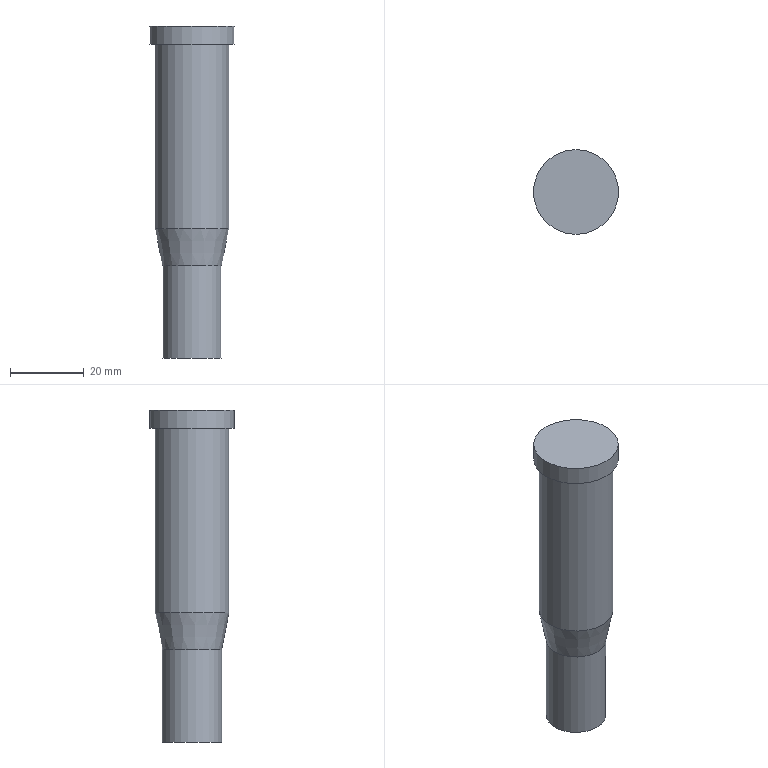Part | NX | features solid 2 | 1 solid | 7 faces | box 23 x 23 x 90 mm | volume 25444 mm3 | plane 3 | cylinder 3 | cone 1 | commonest cylinder face diameters 16.1 x1 20 x1 23 x1
STEP:
#1=CARTESIAN_POINT('',(-384.,15.95,111.));
#2=VERTEX_POINT('',#1);
#3=CARTESIAN_POINT('',(-384.,24.,111.));
#4=DIRECTION('',(0.,0.,1.));
#5=DIRECTION('',(0.,-1.,0.));
#6=AXIS2_PLACEMENT_3D('',#3,#4,#5);
#7=CIRCLE('',#6,8.05);
#8=EDGE_CURVE('',#2,#2,#7,.T.);
#9=ORIENTED_EDGE('',*,*,#8,.F.);
#10=EDGE_LOOP('',(#9));
#11=FACE_BOUND('',#10,.T.);
#12=CARTESIAN_POINT('',(-384.,24.,111.));
#13=DIRECTION('',(0.,0.,-1.));
#14=DIRECTION('',(0.,1.,0.));
#15=AXIS2_PLACEMENT_3D('',#12,#13,#14);
#16=PLANE('',#15);
#17=ADVANCED_FACE('',(#11),#16,.T.);
#18=CARTESIAN_POINT('',(-384.,15.95,136.));
#19=VERTEX_POINT('',#18);
#20=CARTESIAN_POINT('',(-384.,24.,136.));
#21=DIRECTION('',(0.,0.,1.));
#22=DIRECTION('',(0.,-1.,0.));
#23=AXIS2_PLACEMENT_3D('',#20,#21,#22);
#24=CIRCLE('',#23,8.05);
#25=EDGE_CURVE('',#19,#19,#24,.T.);
#26=ORIENTED_EDGE('',*,*,#25,.F.);
#27=EDGE_LOOP('',(#26));
#28=FACE_BOUND('',#27,.T.);
#29=ORIENTED_EDGE('',*,*,#8,.T.);
#30=EDGE_LOOP('',(#29));
#31=FACE_BOUND('',#30,.T.);
#32=CARTESIAN_POINT('',(-384.,24.,111.));
#33=DIRECTION('',(0.,0.,1.));
#34=DIRECTION('',(0.,-1.,0.));
#35=AXIS2_PLACEMENT_3D('',#32,#33,#34);
#36=CYLINDRICAL_SURFACE('',#35,8.05);
#37=ADVANCED_FACE('',(#28,#31),#36,.T.);
#38=ORIENTED_EDGE('',*,*,#25,.T.);
#39=EDGE_LOOP('',(#38));
#40=FACE_BOUND('',#39,.T.);
#41=CARTESIAN_POINT('',(-384.,14.,146.));
#42=VERTEX_POINT('',#41);
#43=CARTESIAN_POINT('',(-384.,24.,146.));
#44=DIRECTION('',(0.,0.,1.));
#45=DIRECTION('',(0.,-1.,0.));
#46=AXIS2_PLACEMENT_3D('',#43,#44,#45);
#47=CIRCLE('',#46,10.);
#48=EDGE_CURVE('',#42,#42,#47,.T.);
#49=ORIENTED_EDGE('',*,*,#48,.F.);
#50=EDGE_LOOP('',(#49));
#51=FACE_BOUND('',#50,.T.);
#52=CARTESIAN_POINT('',(-384.,24.,136.));
#53=DIRECTION('',(0.,0.,1.));
#54=DIRECTION('',(0.,-1.,0.));
#55=AXIS2_PLACEMENT_3D('',#52,#53,#54);
#56=CONICAL_SURFACE('',#55,8.05,0.1926);
#57=ADVANCED_FACE('',(#40,#51),#56,.T.);
#58=CARTESIAN_POINT('',(-384.,34.,196.));
#59=VERTEX_POINT('',#58);
#60=CARTESIAN_POINT('',(-384.,24.,196.));
#61=DIRECTION('',(0.,0.,-1.));
#62=DIRECTION('',(0.,1.,0.));
#63=AXIS2_PLACEMENT_3D('',#60,#61,#62);
#64=CIRCLE('',#63,10.);
#65=EDGE_CURVE('',#59,#59,#64,.F.);
#66=ORIENTED_EDGE('',*,*,#65,.F.);
#67=EDGE_LOOP('',(#66));
#68=FACE_BOUND('',#67,.T.);
#69=ORIENTED_EDGE('',*,*,#48,.T.);
#70=EDGE_LOOP('',(#69));
#71=FACE_BOUND('',#70,.T.);
#72=CARTESIAN_POINT('',(-384.,24.,146.));
#73=DIRECTION('',(0.,0.,1.));
#74=DIRECTION('',(0.,-1.,0.));
#75=AXIS2_PLACEMENT_3D('',#72,#73,#74);
#76=CYLINDRICAL_SURFACE('',#75,10.);
#77=ADVANCED_FACE('',(#68,#71),#76,.T.);
#78=CARTESIAN_POINT('',(-384.,12.5,201.));
#79=VERTEX_POINT('',#78);
#80=CARTESIAN_POINT('',(-384.,24.,201.));
#81=DIRECTION('',(0.,0.,1.));
#82=DIRECTION('',(0.,-1.,0.));
#83=AXIS2_PLACEMENT_3D('',#80,#81,#82);
#84=CIRCLE('',#83,11.5);
#85=EDGE_CURVE('',#79,#79,#84,.F.);
#86=ORIENTED_EDGE('',*,*,#85,.F.);
#87=EDGE_LOOP('',(#86));
#88=FACE_BOUND('',#87,.T.);
#89=CARTESIAN_POINT('',(-384.,24.,201.));
#90=DIRECTION('',(0.,0.,1.));
#91=DIRECTION('',(0.,-1.,0.));
#92=AXIS2_PLACEMENT_3D('',#89,#90,#91);
#93=PLANE('',#92);
#94=ADVANCED_FACE('',(#88),#93,.T.);
#95=ORIENTED_EDGE('',*,*,#65,.T.);
#96=EDGE_LOOP('',(#95));
#97=FACE_BOUND('',#96,.T.);
#98=CARTESIAN_POINT('',(-384.,35.5,196.));
#99=VERTEX_POINT('',#98);
#100=CARTESIAN_POINT('',(-384.,24.,196.));
#101=DIRECTION('',(0.,0.,-1.));
#102=DIRECTION('',(0.,1.,0.));
#103=AXIS2_PLACEMENT_3D('',#100,#101,#102);
#104=CIRCLE('',#103,11.5);
#105=EDGE_CURVE('',#99,#99,#104,.F.);
#106=ORIENTED_EDGE('',*,*,#105,.F.);
#107=EDGE_LOOP('',(#106));
#108=FACE_BOUND('',#107,.T.);
#109=CARTESIAN_POINT('',(-384.,24.,196.));
#110=DIRECTION('',(0.,0.,-1.));
#111=DIRECTION('',(0.,1.,0.));
#112=AXIS2_PLACEMENT_3D('',#109,#110,#111);
#113=PLANE('',#112);
#114=ADVANCED_FACE('',(#97,#108),#113,.T.);
#115=ORIENTED_EDGE('',*,*,#85,.T.);
#116=EDGE_LOOP('',(#115));
#117=FACE_BOUND('',#116,.T.);
#118=ORIENTED_EDGE('',*,*,#105,.T.);
#119=EDGE_LOOP('',(#118));
#120=FACE_BOUND('',#119,.T.);
#121=CARTESIAN_POINT('',(-384.,24.,186.));
#122=DIRECTION('',(0.,0.,1.));
#123=DIRECTION('',(0.,-1.,0.));
#124=AXIS2_PLACEMENT_3D('',#121,#122,#123);
#125=CYLINDRICAL_SURFACE('',#124,11.5);
#126=ADVANCED_FACE('',(#117,#120),#125,.T.);
#127=CLOSED_SHELL('',(#17,#37,#57,#77,#94,#114,#126));
#128=MANIFOLD_SOLID_BREP('',#127);
#129=(LENGTH_UNIT()NAMED_UNIT(*)SI_UNIT(.MILLI.,.METRE.));
#130=UNCERTAINTY_MEASURE_WITH_UNIT(LENGTH_MEASURE(0.00001),#129,'','');
#131=(NAMED_UNIT(*)PLANE_ANGLE_UNIT()SI_UNIT($,.RADIAN.));
#132=(NAMED_UNIT(*)SI_UNIT($,.STERADIAN.)SOLID_ANGLE_UNIT());
#133=(GEOMETRIC_REPRESENTATION_CONTEXT(3)GLOBAL_UNCERTAINTY_ASSIGNED_CONTEXT((#130))GLOBAL_UNIT_ASSIGNED_CONTEXT((#129,#131,#132))REPRESENTATION_CONTEXT('',''));
#134=ADVANCED_BREP_SHAPE_REPRESENTATION('',(#128),#133);